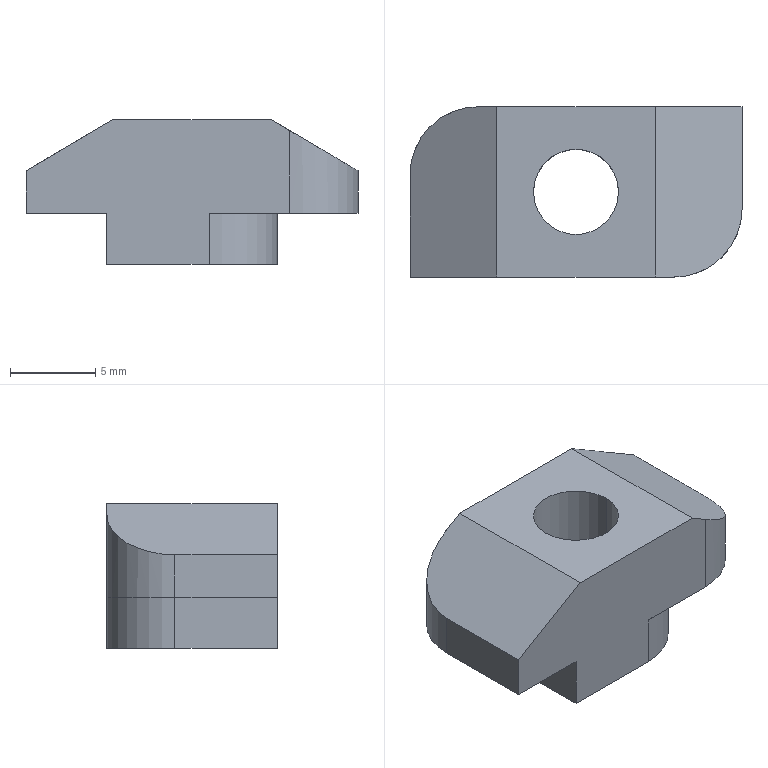Part | NX | features BREP 1 | 1 solid | 18 faces | box 19.5 x 10 x 8.5 mm | volume 1011 mm3 | plane 12 | cylinder 6 | commonest cylinder face diameters 8 x4 5 x2
STEP:
#1=CARTESIAN_POINT('',(-2.5,0.,-8.5));
#2=VERTEX_POINT('',#1);
#3=CARTESIAN_POINT('',(2.5,0.,-8.5));
#4=VERTEX_POINT('',#3);
#5=CARTESIAN_POINT('',(0.,0.,-8.5));
#6=DIRECTION('',(0.,0.,-1.));
#7=DIRECTION('',(-1.,0.,0.));
#8=AXIS2_PLACEMENT_3D('',#5,#6,#7);
#9=CIRCLE('',#8,2.5);
#10=EDGE_CURVE('',#2,#4,#9,.T.);
#11=ORIENTED_EDGE('',*,*,#10,.T.);
#12=CARTESIAN_POINT('',(2.5,0.,0.));
#13=VERTEX_POINT('',#12);
#14=CARTESIAN_POINT('',(2.5,0.,0.));
#15=DIRECTION('',(0.,0.,1.));
#16=VECTOR('',#15,1000.);
#17=LINE('',#14,#16);
#18=EDGE_CURVE('',#4,#13,#17,.T.);
#19=ORIENTED_EDGE('',*,*,#18,.T.);
#20=CARTESIAN_POINT('',(-2.5,0.,0.));
#21=VERTEX_POINT('',#20);
#22=CARTESIAN_POINT('',(0.,0.,0.));
#23=DIRECTION('',(0.,0.,-1.));
#24=DIRECTION('',(-1.,0.,0.));
#25=AXIS2_PLACEMENT_3D('',#22,#23,#24);
#26=CIRCLE('',#25,2.5);
#27=EDGE_CURVE('',#21,#13,#26,.T.);
#28=ORIENTED_EDGE('',*,*,#27,.F.);
#29=CARTESIAN_POINT('',(-2.5,0.,0.));
#30=DIRECTION('',(0.,0.,1.));
#31=VECTOR('',#30,1000.);
#32=LINE('',#29,#31);
#33=EDGE_CURVE('',#2,#21,#32,.T.);
#34=ORIENTED_EDGE('',*,*,#33,.F.);
#35=EDGE_LOOP('',(#11,#19,#28,#34));
#36=FACE_BOUND('',#35,.T.);
#37=CARTESIAN_POINT('',(0.,0.,0.));
#38=DIRECTION('',(0.,0.,1.));
#39=DIRECTION('',(-1.,0.,0.));
#40=AXIS2_PLACEMENT_3D('',#37,#38,#39);
#41=CYLINDRICAL_SURFACE('',#40,2.5);
#42=ADVANCED_FACE('',(#36),#41,.F.);
#43=CARTESIAN_POINT('',(1.,-5.,-5.5));
#44=VERTEX_POINT('',#43);
#45=CARTESIAN_POINT('',(5.75,-5.,-5.5));
#46=VERTEX_POINT('',#45);
#47=CARTESIAN_POINT('',(-9.75,-5.,-5.5));
#48=DIRECTION('',(1.,0.,0.));
#49=VECTOR('',#48,1000.);
#50=LINE('',#47,#49);
#51=EDGE_CURVE('',#44,#46,#50,.T.);
#52=ORIENTED_EDGE('',*,*,#51,.F.);
#53=CARTESIAN_POINT('',(5.,-1.,-5.5));
#54=VERTEX_POINT('',#53);
#55=CARTESIAN_POINT('',(1.,-1.,-5.5));
#56=DIRECTION('',(0.,0.,-1.));
#57=DIRECTION('',(1.,0.,0.));
#58=AXIS2_PLACEMENT_3D('',#55,#56,#57);
#59=CIRCLE('',#58,4.);
#60=EDGE_CURVE('',#54,#44,#59,.T.);
#61=ORIENTED_EDGE('',*,*,#60,.F.);
#62=CARTESIAN_POINT('',(5.,5.,-5.5));
#63=VERTEX_POINT('',#62);
#64=CARTESIAN_POINT('',(5.,-5.,-5.5));
#65=DIRECTION('',(0.,1.,0.));
#66=VECTOR('',#65,1000.);
#67=LINE('',#64,#66);
#68=EDGE_CURVE('',#54,#63,#67,.T.);
#69=ORIENTED_EDGE('',*,*,#68,.T.);
#70=CARTESIAN_POINT('',(9.75,5.,-5.5));
#71=VERTEX_POINT('',#70);
#72=CARTESIAN_POINT('',(-9.75,5.,-5.5));
#73=DIRECTION('',(-1.,0.,0.));
#74=VECTOR('',#73,1000.);
#75=LINE('',#72,#74);
#76=EDGE_CURVE('',#71,#63,#75,.T.);
#77=ORIENTED_EDGE('',*,*,#76,.F.);
#78=CARTESIAN_POINT('',(9.75,-1.,-5.5));
#79=VERTEX_POINT('',#78);
#80=CARTESIAN_POINT('',(9.75,5.,-5.5));
#81=DIRECTION('',(0.,1.,0.));
#82=VECTOR('',#81,1000.);
#83=LINE('',#80,#82);
#84=EDGE_CURVE('',#79,#71,#83,.T.);
#85=ORIENTED_EDGE('',*,*,#84,.F.);
#86=CARTESIAN_POINT('',(5.75,-1.,-5.5));
#87=DIRECTION('',(0.,0.,1.));
#88=DIRECTION('',(1.,0.,0.));
#89=AXIS2_PLACEMENT_3D('',#86,#87,#88);
#90=CIRCLE('',#89,4.);
#91=EDGE_CURVE('',#46,#79,#90,.T.);
#92=ORIENTED_EDGE('',*,*,#91,.F.);
#93=EDGE_LOOP('',(#52,#61,#69,#77,#85,#92));
#94=FACE_BOUND('',#93,.T.);
#95=CARTESIAN_POINT('',(0.,0.,-5.5));
#96=DIRECTION('',(0.,0.,-1.));
#97=DIRECTION('',(0.,-1.,0.));
#98=AXIS2_PLACEMENT_3D('',#95,#96,#97);
#99=PLANE('',#98);
#100=ADVANCED_FACE('',(#94),#99,.T.);
#101=ORIENTED_EDGE('',*,*,#84,.T.);
#102=CARTESIAN_POINT('',(9.75,5.,-3.));
#103=VERTEX_POINT('',#102);
#104=CARTESIAN_POINT('',(9.75,5.,-5.5));
#105=DIRECTION('',(0.,0.,1.));
#106=VECTOR('',#105,1000.);
#107=LINE('',#104,#106);
#108=EDGE_CURVE('',#71,#103,#107,.T.);
#109=ORIENTED_EDGE('',*,*,#108,.T.);
#110=CARTESIAN_POINT('',(9.75,-1.,-3.));
#111=VERTEX_POINT('',#110);
#112=CARTESIAN_POINT('',(9.75,5.,-3.));
#113=DIRECTION('',(0.,1.,0.));
#114=VECTOR('',#113,1000.);
#115=LINE('',#112,#114);
#116=EDGE_CURVE('',#111,#103,#115,.T.);
#117=ORIENTED_EDGE('',*,*,#116,.F.);
#118=CARTESIAN_POINT('',(9.75,-1.,-5.5));
#119=DIRECTION('',(0.,0.,1.));
#120=VECTOR('',#119,1000.);
#121=LINE('',#118,#120);
#122=EDGE_CURVE('',#79,#111,#121,.T.);
#123=ORIENTED_EDGE('',*,*,#122,.F.);
#124=EDGE_LOOP('',(#101,#109,#117,#123));
#125=FACE_BOUND('',#124,.T.);
#126=CARTESIAN_POINT('',(9.75,5.,-5.5));
#127=DIRECTION('',(-1.,0.,0.));
#128=DIRECTION('',(0.,1.,0.));
#129=AXIS2_PLACEMENT_3D('',#126,#127,#128);
#130=PLANE('',#129);
#131=ADVANCED_FACE('',(#125),#130,.F.);
#132=CARTESIAN_POINT('',(-4.65,5.,0.));
#133=VERTEX_POINT('',#132);
#134=CARTESIAN_POINT('',(-5.75,5.,-0.6471));
#135=VERTEX_POINT('',#134);
#136=CARTESIAN_POINT('',(-9.75,5.,-3.));
#137=DIRECTION('',(-0.8619,0.,-0.507));
#138=VECTOR('',#137,1000.);
#139=LINE('',#136,#138);
#140=EDGE_CURVE('',#133,#135,#139,.T.);
#141=ORIENTED_EDGE('',*,*,#140,.F.);
#142=CARTESIAN_POINT('',(4.65,5.,0.));
#143=VERTEX_POINT('',#142);
#144=CARTESIAN_POINT('',(-9.75,5.,0.));
#145=DIRECTION('',(-1.,0.,0.));
#146=VECTOR('',#145,1000.);
#147=LINE('',#144,#146);
#148=EDGE_CURVE('',#143,#133,#147,.T.);
#149=ORIENTED_EDGE('',*,*,#148,.F.);
#150=CARTESIAN_POINT('',(9.75,5.,-3.));
#151=DIRECTION('',(-0.8619,0.,0.507));
#152=VECTOR('',#151,1000.);
#153=LINE('',#150,#152);
#154=EDGE_CURVE('',#103,#143,#153,.T.);
#155=ORIENTED_EDGE('',*,*,#154,.F.);
#156=ORIENTED_EDGE('',*,*,#108,.F.);
#157=ORIENTED_EDGE('',*,*,#76,.T.);
#158=CARTESIAN_POINT('',(5.,5.,-8.5));
#159=VERTEX_POINT('',#158);
#160=CARTESIAN_POINT('',(5.,5.,-8.5));
#161=DIRECTION('',(0.,0.,1.));
#162=VECTOR('',#161,1000.);
#163=LINE('',#160,#162);
#164=EDGE_CURVE('',#159,#63,#163,.T.);
#165=ORIENTED_EDGE('',*,*,#164,.F.);
#166=CARTESIAN_POINT('',(-1.,5.,-8.5));
#167=VERTEX_POINT('',#166);
#168=CARTESIAN_POINT('',(-5.,5.,-8.5));
#169=DIRECTION('',(-1.,0.,0.));
#170=VECTOR('',#169,1000.);
#171=LINE('',#168,#170);
#172=EDGE_CURVE('',#159,#167,#171,.T.);
#173=ORIENTED_EDGE('',*,*,#172,.T.);
#174=CARTESIAN_POINT('',(-1.,5.,-5.5));
#175=VERTEX_POINT('',#174);
#176=CARTESIAN_POINT('',(-1.,5.,-5.5));
#177=DIRECTION('',(0.,0.,-1.));
#178=VECTOR('',#177,1000.);
#179=LINE('',#176,#178);
#180=EDGE_CURVE('',#175,#167,#179,.T.);
#181=ORIENTED_EDGE('',*,*,#180,.F.);
#182=CARTESIAN_POINT('',(-5.75,5.,-5.5));
#183=VERTEX_POINT('',#182);
#184=CARTESIAN_POINT('',(-9.75,5.,-5.5));
#185=DIRECTION('',(-1.,0.,0.));
#186=VECTOR('',#185,1000.);
#187=LINE('',#184,#186);
#188=EDGE_CURVE('',#175,#183,#187,.T.);
#189=ORIENTED_EDGE('',*,*,#188,.T.);
#190=CARTESIAN_POINT('',(-5.75,5.,-5.5));
#191=DIRECTION('',(0.,0.,-1.));
#192=VECTOR('',#191,1000.);
#193=LINE('',#190,#192);
#194=EDGE_CURVE('',#135,#183,#193,.T.);
#195=ORIENTED_EDGE('',*,*,#194,.F.);
#196=EDGE_LOOP('',(#141,#149,#155,#156,#157,#165,#173,#181,#189,#195));
#197=FACE_BOUND('',#196,.T.);
#198=CARTESIAN_POINT('',(-9.75,5.,-5.5));
#199=DIRECTION('',(0.,-1.,0.));
#200=DIRECTION('',(0.,0.,-1.));
#201=AXIS2_PLACEMENT_3D('',#198,#199,#200);
#202=PLANE('',#201);
#203=ADVANCED_FACE('',(#197),#202,.F.);
#204=CARTESIAN_POINT('',(-9.75,1.,-5.5));
#205=VERTEX_POINT('',#204);
#206=CARTESIAN_POINT('',(-9.75,-5.,-5.5));
#207=VERTEX_POINT('',#206);
#208=CARTESIAN_POINT('',(-9.75,5.,-5.5));
#209=DIRECTION('',(0.,-1.,0.));
#210=VECTOR('',#209,1000.);
#211=LINE('',#208,#210);
#212=EDGE_CURVE('',#205,#207,#211,.T.);
#213=ORIENTED_EDGE('',*,*,#212,.T.);
#214=CARTESIAN_POINT('',(-9.75,-5.,-3.));
#215=VERTEX_POINT('',#214);
#216=CARTESIAN_POINT('',(-9.75,-5.,-5.5));
#217=DIRECTION('',(0.,0.,1.));
#218=VECTOR('',#217,1000.);
#219=LINE('',#216,#218);
#220=EDGE_CURVE('',#207,#215,#219,.T.);
#221=ORIENTED_EDGE('',*,*,#220,.T.);
#222=CARTESIAN_POINT('',(-9.75,1.,-3.));
#223=VERTEX_POINT('',#222);
#224=CARTESIAN_POINT('',(-9.75,5.,-3.));
#225=DIRECTION('',(0.,-1.,0.));
#226=VECTOR('',#225,1000.);
#227=LINE('',#224,#226);
#228=EDGE_CURVE('',#223,#215,#227,.T.);
#229=ORIENTED_EDGE('',*,*,#228,.F.);
#230=CARTESIAN_POINT('',(-9.75,1.,-5.5));
#231=DIRECTION('',(0.,0.,1.));
#232=VECTOR('',#231,1000.);
#233=LINE('',#230,#232);
#234=EDGE_CURVE('',#205,#223,#233,.T.);
#235=ORIENTED_EDGE('',*,*,#234,.F.);
#236=EDGE_LOOP('',(#213,#221,#229,#235));
#237=FACE_BOUND('',#236,.T.);
#238=CARTESIAN_POINT('',(-9.75,5.,-5.5));
#239=DIRECTION('',(1.,0.,0.));
#240=DIRECTION('',(0.,1.,0.));
#241=AXIS2_PLACEMENT_3D('',#238,#239,#240);
#242=PLANE('',#241);
#243=ADVANCED_FACE('',(#237),#242,.F.);
#244=CARTESIAN_POINT('',(4.65,-5.,0.));
#245=VERTEX_POINT('',#244);
#246=CARTESIAN_POINT('',(5.75,-5.,-0.6471));
#247=VERTEX_POINT('',#246);
#248=CARTESIAN_POINT('',(9.75,-5.,-3.));
#249=DIRECTION('',(0.8619,0.,-0.507));
#250=VECTOR('',#249,1000.);
#251=LINE('',#248,#250);
#252=EDGE_CURVE('',#245,#247,#251,.T.);
#253=ORIENTED_EDGE('',*,*,#252,.F.);
#254=CARTESIAN_POINT('',(-4.65,-5.,0.));
#255=VERTEX_POINT('',#254);
#256=CARTESIAN_POINT('',(-9.75,-5.,0.));
#257=DIRECTION('',(1.,0.,0.));
#258=VECTOR('',#257,1000.);
#259=LINE('',#256,#258);
#260=EDGE_CURVE('',#255,#245,#259,.T.);
#261=ORIENTED_EDGE('',*,*,#260,.F.);
#262=CARTESIAN_POINT('',(-9.75,-5.,-3.));
#263=DIRECTION('',(0.8619,0.,0.507));
#264=VECTOR('',#263,1000.);
#265=LINE('',#262,#264);
#266=EDGE_CURVE('',#215,#255,#265,.T.);
#267=ORIENTED_EDGE('',*,*,#266,.F.);
#268=ORIENTED_EDGE('',*,*,#220,.F.);
#269=CARTESIAN_POINT('',(-5.,-5.,-5.5));
#270=VERTEX_POINT('',#269);
#271=CARTESIAN_POINT('',(-9.75,-5.,-5.5));
#272=DIRECTION('',(1.,0.,0.));
#273=VECTOR('',#272,1000.);
#274=LINE('',#271,#273);
#275=EDGE_CURVE('',#207,#270,#274,.T.);
#276=ORIENTED_EDGE('',*,*,#275,.T.);
#277=CARTESIAN_POINT('',(-5.,-5.,-8.5));
#278=VERTEX_POINT('',#277);
#279=CARTESIAN_POINT('',(-5.,-5.,-8.5));
#280=DIRECTION('',(0.,0.,1.));
#281=VECTOR('',#280,1000.);
#282=LINE('',#279,#281);
#283=EDGE_CURVE('',#278,#270,#282,.T.);
#284=ORIENTED_EDGE('',*,*,#283,.F.);
#285=CARTESIAN_POINT('',(1.,-5.,-8.5));
#286=VERTEX_POINT('',#285);
#287=CARTESIAN_POINT('',(-5.,-5.,-8.5));
#288=DIRECTION('',(1.,0.,0.));
#289=VECTOR('',#288,1000.);
#290=LINE('',#287,#289);
#291=EDGE_CURVE('',#278,#286,#290,.T.);
#292=ORIENTED_EDGE('',*,*,#291,.T.);
#293=CARTESIAN_POINT('',(1.,-5.,-5.5));
#294=DIRECTION('',(0.,0.,-1.));
#295=VECTOR('',#294,1000.);
#296=LINE('',#293,#295);
#297=EDGE_CURVE('',#44,#286,#296,.T.);
#298=ORIENTED_EDGE('',*,*,#297,.F.);
#299=ORIENTED_EDGE('',*,*,#51,.T.);
#300=CARTESIAN_POINT('',(5.75,-5.,-5.5));
#301=DIRECTION('',(0.,0.,-1.));
#302=VECTOR('',#301,1000.);
#303=LINE('',#300,#302);
#304=EDGE_CURVE('',#247,#46,#303,.T.);
#305=ORIENTED_EDGE('',*,*,#304,.F.);
#306=EDGE_LOOP('',(#253,#261,#267,#268,#276,#284,#292,#298,#299,#305));
#307=FACE_BOUND('',#306,.T.);
#308=CARTESIAN_POINT('',(-9.75,-5.,-5.5));
#309=DIRECTION('',(0.,1.,0.));
#310=DIRECTION('',(1.,0.,0.));
#311=AXIS2_PLACEMENT_3D('',#308,#309,#310);
#312=PLANE('',#311);
#313=ADVANCED_FACE('',(#307),#312,.F.);
#314=ORIENTED_EDGE('',*,*,#188,.F.);
#315=CARTESIAN_POINT('',(-5.,1.,-5.5));
#316=VERTEX_POINT('',#315);
#317=CARTESIAN_POINT('',(-1.,1.,-5.5));
#318=DIRECTION('',(0.,0.,-1.));
#319=DIRECTION('',(1.,0.,0.));
#320=AXIS2_PLACEMENT_3D('',#317,#318,#319);
#321=CIRCLE('',#320,4.);
#322=EDGE_CURVE('',#316,#175,#321,.T.);
#323=ORIENTED_EDGE('',*,*,#322,.F.);
#324=CARTESIAN_POINT('',(-5.,-5.,-5.5));
#325=DIRECTION('',(0.,-1.,0.));
#326=VECTOR('',#325,1000.);
#327=LINE('',#324,#326);
#328=EDGE_CURVE('',#316,#270,#327,.T.);
#329=ORIENTED_EDGE('',*,*,#328,.T.);
#330=ORIENTED_EDGE('',*,*,#275,.F.);
#331=ORIENTED_EDGE('',*,*,#212,.F.);
#332=CARTESIAN_POINT('',(-5.75,1.,-5.5));
#333=DIRECTION('',(0.,0.,1.));
#334=DIRECTION('',(1.,0.,0.));
#335=AXIS2_PLACEMENT_3D('',#332,#333,#334);
#336=CIRCLE('',#335,4.);
#337=EDGE_CURVE('',#183,#205,#336,.T.);
#338=ORIENTED_EDGE('',*,*,#337,.F.);
#339=EDGE_LOOP('',(#314,#323,#329,#330,#331,#338));
#340=FACE_BOUND('',#339,.T.);
#341=CARTESIAN_POINT('',(0.,0.,-5.5));
#342=DIRECTION('',(0.,0.,-1.));
#343=DIRECTION('',(0.,-1.,0.));
#344=AXIS2_PLACEMENT_3D('',#341,#342,#343);
#345=PLANE('',#344);
#346=ADVANCED_FACE('',(#340),#345,.T.);
#347=ORIENTED_EDGE('',*,*,#148,.T.);
#348=CARTESIAN_POINT('',(-4.65,0.,0.));
#349=DIRECTION('',(0.,1.,0.));
#350=VECTOR('',#349,1000.);
#351=LINE('',#348,#350);
#352=EDGE_CURVE('',#255,#133,#351,.T.);
#353=ORIENTED_EDGE('',*,*,#352,.F.);
#354=ORIENTED_EDGE('',*,*,#260,.T.);
#355=CARTESIAN_POINT('',(4.65,0.,0.));
#356=DIRECTION('',(0.,-1.,0.));
#357=VECTOR('',#356,1000.);
#358=LINE('',#355,#357);
#359=EDGE_CURVE('',#143,#245,#358,.T.);
#360=ORIENTED_EDGE('',*,*,#359,.F.);
#361=EDGE_LOOP('',(#347,#353,#354,#360));
#362=FACE_BOUND('',#361,.T.);
#363=ORIENTED_EDGE('',*,*,#27,.T.);
#364=CARTESIAN_POINT('',(0.,0.,0.));
#365=DIRECTION('',(0.,0.,-1.));
#366=DIRECTION('',(-1.,0.,0.));
#367=AXIS2_PLACEMENT_3D('',#364,#365,#366);
#368=CIRCLE('',#367,2.5);
#369=EDGE_CURVE('',#13,#21,#368,.T.);
#370=ORIENTED_EDGE('',*,*,#369,.T.);
#371=EDGE_LOOP('',(#363,#370));
#372=FACE_BOUND('',#371,.T.);
#373=CARTESIAN_POINT('',(0.,0.,0.));
#374=DIRECTION('',(0.,0.,-1.));
#375=DIRECTION('',(0.,-1.,0.));
#376=AXIS2_PLACEMENT_3D('',#373,#374,#375);
#377=PLANE('',#376);
#378=ADVANCED_FACE('',(#362,#372),#377,.F.);
#379=CARTESIAN_POINT('',(5.,-1.,-8.5));
#380=VERTEX_POINT('',#379);
#381=CARTESIAN_POINT('',(5.,-5.,-8.5));
#382=DIRECTION('',(0.,1.,0.));
#383=VECTOR('',#382,1000.);
#384=LINE('',#381,#383);
#385=EDGE_CURVE('',#380,#159,#384,.T.);
#386=ORIENTED_EDGE('',*,*,#385,.T.);
#387=ORIENTED_EDGE('',*,*,#164,.T.);
#388=ORIENTED_EDGE('',*,*,#68,.F.);
#389=CARTESIAN_POINT('',(5.,-1.,-8.5));
#390=DIRECTION('',(0.,0.,1.));
#391=VECTOR('',#390,1000.);
#392=LINE('',#389,#391);
#393=EDGE_CURVE('',#380,#54,#392,.T.);
#394=ORIENTED_EDGE('',*,*,#393,.F.);
#395=EDGE_LOOP('',(#386,#387,#388,#394));
#396=FACE_BOUND('',#395,.T.);
#397=CARTESIAN_POINT('',(5.,-5.,-8.5));
#398=DIRECTION('',(-1.,0.,0.));
#399=DIRECTION('',(0.,0.,1.));
#400=AXIS2_PLACEMENT_3D('',#397,#398,#399);
#401=PLANE('',#400);
#402=ADVANCED_FACE('',(#396),#401,.F.);
#403=CARTESIAN_POINT('',(-5.,1.,-8.5));
#404=VERTEX_POINT('',#403);
#405=CARTESIAN_POINT('',(-5.,-5.,-8.5));
#406=DIRECTION('',(0.,-1.,0.));
#407=VECTOR('',#406,1000.);
#408=LINE('',#405,#407);
#409=EDGE_CURVE('',#404,#278,#408,.T.);
#410=ORIENTED_EDGE('',*,*,#409,.T.);
#411=ORIENTED_EDGE('',*,*,#283,.T.);
#412=ORIENTED_EDGE('',*,*,#328,.F.);
#413=CARTESIAN_POINT('',(-5.,1.,-8.5));
#414=DIRECTION('',(0.,0.,1.));
#415=VECTOR('',#414,1000.);
#416=LINE('',#413,#415);
#417=EDGE_CURVE('',#404,#316,#416,.T.);
#418=ORIENTED_EDGE('',*,*,#417,.F.);
#419=EDGE_LOOP('',(#410,#411,#412,#418));
#420=FACE_BOUND('',#419,.T.);
#421=CARTESIAN_POINT('',(-5.,-5.,-8.5));
#422=DIRECTION('',(1.,0.,0.));
#423=DIRECTION('',(0.,1.,0.));
#424=AXIS2_PLACEMENT_3D('',#421,#422,#423);
#425=PLANE('',#424);
#426=ADVANCED_FACE('',(#420),#425,.F.);
#427=ORIENTED_EDGE('',*,*,#291,.F.);
#428=ORIENTED_EDGE('',*,*,#409,.F.);
#429=CARTESIAN_POINT('',(-1.,1.,-8.5));
#430=DIRECTION('',(0.,0.,1.));
#431=DIRECTION('',(-1.,0.,0.));
#432=AXIS2_PLACEMENT_3D('',#429,#430,#431);
#433=CIRCLE('',#432,4.);
#434=EDGE_CURVE('',#167,#404,#433,.T.);
#435=ORIENTED_EDGE('',*,*,#434,.F.);
#436=ORIENTED_EDGE('',*,*,#172,.F.);
#437=ORIENTED_EDGE('',*,*,#385,.F.);
#438=CARTESIAN_POINT('',(1.,-1.,-8.5));
#439=DIRECTION('',(0.,0.,1.));
#440=DIRECTION('',(-1.,0.,0.));
#441=AXIS2_PLACEMENT_3D('',#438,#439,#440);
#442=CIRCLE('',#441,4.);
#443=EDGE_CURVE('',#286,#380,#442,.T.);
#444=ORIENTED_EDGE('',*,*,#443,.F.);
#445=EDGE_LOOP('',(#427,#428,#435,#436,#437,#444));
#446=FACE_BOUND('',#445,.T.);
#447=ORIENTED_EDGE('',*,*,#10,.F.);
#448=CARTESIAN_POINT('',(0.,0.,-8.5));
#449=DIRECTION('',(0.,0.,-1.));
#450=DIRECTION('',(-1.,0.,0.));
#451=AXIS2_PLACEMENT_3D('',#448,#449,#450);
#452=CIRCLE('',#451,2.5);
#453=EDGE_CURVE('',#4,#2,#452,.T.);
#454=ORIENTED_EDGE('',*,*,#453,.F.);
#455=EDGE_LOOP('',(#447,#454));
#456=FACE_BOUND('',#455,.T.);
#457=CARTESIAN_POINT('',(0.,0.,-8.5));
#458=DIRECTION('',(0.,0.,1.));
#459=DIRECTION('',(1.,0.,0.));
#460=AXIS2_PLACEMENT_3D('',#457,#458,#459);
#461=PLANE('',#460);
#462=ADVANCED_FACE('',(#446,#456),#461,.F.);
#463=ORIENTED_EDGE('',*,*,#18,.F.);
#464=ORIENTED_EDGE('',*,*,#453,.T.);
#465=ORIENTED_EDGE('',*,*,#33,.T.);
#466=ORIENTED_EDGE('',*,*,#369,.F.);
#467=EDGE_LOOP('',(#463,#464,#465,#466));
#468=FACE_BOUND('',#467,.T.);
#469=CARTESIAN_POINT('',(0.,0.,0.));
#470=DIRECTION('',(0.,0.,1.));
#471=DIRECTION('',(-1.,0.,0.));
#472=AXIS2_PLACEMENT_3D('',#469,#470,#471);
#473=CYLINDRICAL_SURFACE('',#472,2.5);
#474=ADVANCED_FACE('',(#468),#473,.F.);
#475=ORIENTED_EDGE('',*,*,#116,.T.);
#476=ORIENTED_EDGE('',*,*,#154,.T.);
#477=ORIENTED_EDGE('',*,*,#359,.T.);
#478=ORIENTED_EDGE('',*,*,#252,.T.);
#479=CARTESIAN_POINT('',(9.75,-1.,-3.));
#480=CARTESIAN_POINT('',(9.75,-3.343,-3.));
#481=CARTESIAN_POINT('',(8.093,-5.,-2.025));
#482=CARTESIAN_POINT('',(5.75,-5.,-0.6471));
#483=(BOUNDED_CURVE()B_SPLINE_CURVE(3,(#479,#480,#481,#482),.UNSPECIFIED.,.F.,.F.)B_SPLINE_CURVE_WITH_KNOTS((4,4),(3.142,4.712),.UNSPECIFIED.)CURVE()GEOMETRIC_REPRESENTATION_ITEM()RATIONAL_B_SPLINE_CURVE((1.,0.8047,0.8047,1.))REPRESENTATION_ITEM(''));
#484=EDGE_CURVE('',#111,#247,#483,.T.);
#485=ORIENTED_EDGE('',*,*,#484,.F.);
#486=EDGE_LOOP('',(#475,#476,#477,#478,#485));
#487=FACE_BOUND('',#486,.T.);
#488=CARTESIAN_POINT('',(9.75,5.,-3.));
#489=DIRECTION('',(-0.507,0.,-0.8619));
#490=DIRECTION('',(-0.8619,0.,0.507));
#491=AXIS2_PLACEMENT_3D('',#488,#489,#490);
#492=PLANE('',#491);
#493=ADVANCED_FACE('',(#487),#492,.F.);
#494=ORIENTED_EDGE('',*,*,#228,.T.);
#495=ORIENTED_EDGE('',*,*,#266,.T.);
#496=ORIENTED_EDGE('',*,*,#352,.T.);
#497=ORIENTED_EDGE('',*,*,#140,.T.);
#498=CARTESIAN_POINT('',(-9.75,1.,-3.));
#499=CARTESIAN_POINT('',(-9.75,3.343,-3.));
#500=CARTESIAN_POINT('',(-8.093,5.,-2.025));
#501=CARTESIAN_POINT('',(-5.75,5.,-0.6471));
#502=(BOUNDED_CURVE()B_SPLINE_CURVE(3,(#498,#499,#500,#501),.UNSPECIFIED.,.F.,.F.)B_SPLINE_CURVE_WITH_KNOTS((4,4),(3.142,4.712),.UNSPECIFIED.)CURVE()GEOMETRIC_REPRESENTATION_ITEM()RATIONAL_B_SPLINE_CURVE((1.,0.8047,0.8047,1.))REPRESENTATION_ITEM(''));
#503=EDGE_CURVE('',#223,#135,#502,.T.);
#504=ORIENTED_EDGE('',*,*,#503,.F.);
#505=EDGE_LOOP('',(#494,#495,#496,#497,#504));
#506=FACE_BOUND('',#505,.T.);
#507=CARTESIAN_POINT('',(-9.75,5.,-3.));
#508=DIRECTION('',(0.507,0.,-0.8619));
#509=DIRECTION('',(0.,-1.,0.));
#510=AXIS2_PLACEMENT_3D('',#507,#508,#509);
#511=PLANE('',#510);
#512=ADVANCED_FACE('',(#506),#511,.F.);
#513=ORIENTED_EDGE('',*,*,#443,.T.);
#514=ORIENTED_EDGE('',*,*,#393,.T.);
#515=ORIENTED_EDGE('',*,*,#60,.T.);
#516=ORIENTED_EDGE('',*,*,#297,.T.);
#517=EDGE_LOOP('',(#513,#514,#515,#516));
#518=FACE_BOUND('',#517,.T.);
#519=CARTESIAN_POINT('',(1.,-1.,-8.5));
#520=DIRECTION('',(0.,0.,1.));
#521=DIRECTION('',(-1.,0.,0.));
#522=AXIS2_PLACEMENT_3D('',#519,#520,#521);
#523=CYLINDRICAL_SURFACE('',#522,4.);
#524=ADVANCED_FACE('',(#518),#523,.T.);
#525=ORIENTED_EDGE('',*,*,#434,.T.);
#526=ORIENTED_EDGE('',*,*,#417,.T.);
#527=ORIENTED_EDGE('',*,*,#322,.T.);
#528=ORIENTED_EDGE('',*,*,#180,.T.);
#529=EDGE_LOOP('',(#525,#526,#527,#528));
#530=FACE_BOUND('',#529,.T.);
#531=CARTESIAN_POINT('',(-1.,1.,-8.5));
#532=DIRECTION('',(0.,0.,1.));
#533=DIRECTION('',(-1.,0.,0.));
#534=AXIS2_PLACEMENT_3D('',#531,#532,#533);
#535=CYLINDRICAL_SURFACE('',#534,4.);
#536=ADVANCED_FACE('',(#530),#535,.T.);
#537=ORIENTED_EDGE('',*,*,#91,.T.);
#538=ORIENTED_EDGE('',*,*,#122,.T.);
#539=ORIENTED_EDGE('',*,*,#484,.T.);
#540=ORIENTED_EDGE('',*,*,#304,.T.);
#541=EDGE_LOOP('',(#537,#538,#539,#540));
#542=FACE_BOUND('',#541,.T.);
#543=CARTESIAN_POINT('',(5.75,-1.,-5.5));
#544=DIRECTION('',(0.,0.,1.));
#545=DIRECTION('',(-1.,0.,0.));
#546=AXIS2_PLACEMENT_3D('',#543,#544,#545);
#547=CYLINDRICAL_SURFACE('',#546,4.);
#548=ADVANCED_FACE('',(#542),#547,.T.);
#549=ORIENTED_EDGE('',*,*,#337,.T.);
#550=ORIENTED_EDGE('',*,*,#234,.T.);
#551=ORIENTED_EDGE('',*,*,#503,.T.);
#552=ORIENTED_EDGE('',*,*,#194,.T.);
#553=EDGE_LOOP('',(#549,#550,#551,#552));
#554=FACE_BOUND('',#553,.T.);
#555=CARTESIAN_POINT('',(-5.75,1.,-5.5));
#556=DIRECTION('',(0.,0.,1.));
#557=DIRECTION('',(-1.,0.,0.));
#558=AXIS2_PLACEMENT_3D('',#555,#556,#557);
#559=CYLINDRICAL_SURFACE('',#558,4.);
#560=ADVANCED_FACE('',(#554),#559,.T.);
#561=CLOSED_SHELL('',(#42,#100,#131,#203,#243,#313,#346,#378,#402,#426,#462,#474,#493,#512,#524,#536,#548,#560));
#562=MANIFOLD_SOLID_BREP('',#561);
#563=(LENGTH_UNIT()NAMED_UNIT(*)SI_UNIT(.MILLI.,.METRE.));
#564=UNCERTAINTY_MEASURE_WITH_UNIT(LENGTH_MEASURE(0.00001),#563,'','');
#565=(NAMED_UNIT(*)PLANE_ANGLE_UNIT()SI_UNIT($,.RADIAN.));
#566=(NAMED_UNIT(*)SI_UNIT($,.STERADIAN.)SOLID_ANGLE_UNIT());
#567=(GEOMETRIC_REPRESENTATION_CONTEXT(3)GLOBAL_UNCERTAINTY_ASSIGNED_CONTEXT((#564))GLOBAL_UNIT_ASSIGNED_CONTEXT((#563,#565,#566))REPRESENTATION_CONTEXT('',''));
#568=ADVANCED_BREP_SHAPE_REPRESENTATION('',(#562),#567);